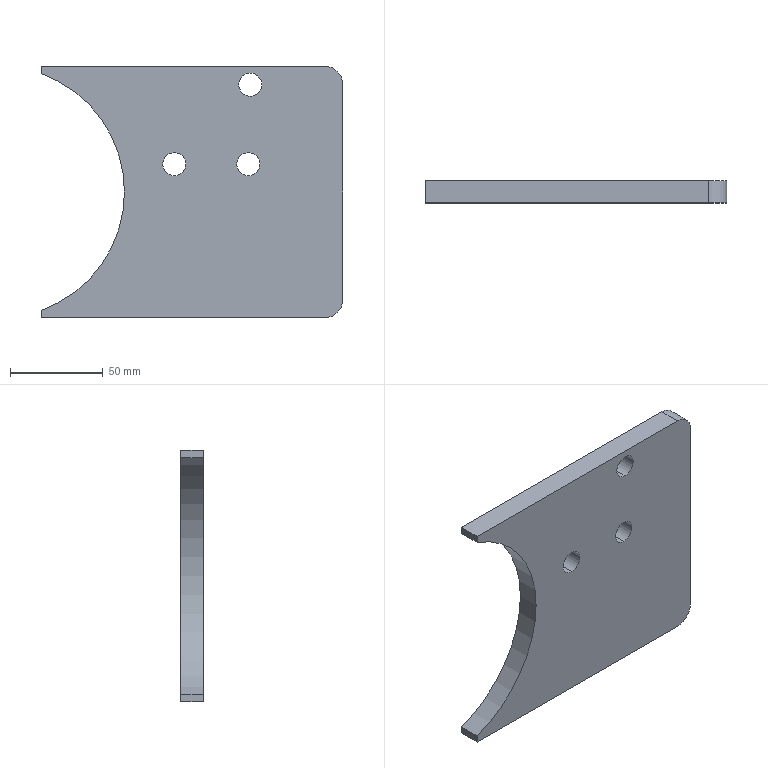Part | SolidWorks | features FlatPattern 1, SMBaseFlange 1, SheetMetal 1 | 1 solid | 16 faces | box 163 x 12 x 136 mm | volume 210730 mm3 | cylinder 9 | plane 7 | commonest cylinder face diameters 12.5 x6 20 x2 136 x1
STEP:
#1=CARTESIAN_POINT('',(113.,-12.,119.75));
#2=VERTEX_POINT('',#1);
#3=CARTESIAN_POINT('',(113.,-12.,132.25));
#4=VERTEX_POINT('',#3);
#5=CARTESIAN_POINT('',(113.,-12.,126.));
#6=DIRECTION('',(0.,1.,0.));
#7=DIRECTION('',(0.,0.,1.));
#8=AXIS2_PLACEMENT_3D('',#5,#6,#7);
#9=CIRCLE('',#8,6.25);
#10=EDGE_CURVE('',#2,#4,#9,.T.);
#11=ORIENTED_EDGE('',*,*,#10,.F.);
#12=CARTESIAN_POINT('',(113.,0.,119.75));
#13=VERTEX_POINT('',#12);
#14=CARTESIAN_POINT('',(113.,-12.,119.75));
#15=DIRECTION('',(0.,1.,0.));
#16=VECTOR('',#15,1000.);
#17=LINE('',#14,#16);
#18=EDGE_CURVE('',#2,#13,#17,.T.);
#19=ORIENTED_EDGE('',*,*,#18,.T.);
#20=CARTESIAN_POINT('',(113.,0.,132.25));
#21=VERTEX_POINT('',#20);
#22=CARTESIAN_POINT('',(113.,0.,126.));
#23=DIRECTION('',(0.,1.,0.));
#24=DIRECTION('',(0.,0.,1.));
#25=AXIS2_PLACEMENT_3D('',#22,#23,#24);
#26=CIRCLE('',#25,6.25);
#27=EDGE_CURVE('',#13,#21,#26,.T.);
#28=ORIENTED_EDGE('',*,*,#27,.T.);
#29=CARTESIAN_POINT('',(113.,-12.,132.25));
#30=DIRECTION('',(0.,1.,0.));
#31=VECTOR('',#30,1000.);
#32=LINE('',#29,#31);
#33=EDGE_CURVE('',#4,#21,#32,.T.);
#34=ORIENTED_EDGE('',*,*,#33,.F.);
#35=EDGE_LOOP('',(#11,#19,#28,#34));
#36=FACE_OUTER_BOUND('',#35,.T.);
#37=CARTESIAN_POINT('',(113.,-12.,126.));
#38=DIRECTION('',(0.,1.,0.));
#39=DIRECTION('',(0.,0.,1.));
#40=AXIS2_PLACEMENT_3D('',#37,#38,#39);
#41=CYLINDRICAL_SURFACE('',#40,6.25);
#42=ADVANCED_FACE('',(#36),#41,.F.);
#43=CARTESIAN_POINT('',(112.,-12.,76.75));
#44=VERTEX_POINT('',#43);
#45=CARTESIAN_POINT('',(112.,-12.,89.25));
#46=VERTEX_POINT('',#45);
#47=CARTESIAN_POINT('',(112.,-12.,83.));
#48=DIRECTION('',(0.,1.,0.));
#49=DIRECTION('',(0.,0.,1.));
#50=AXIS2_PLACEMENT_3D('',#47,#48,#49);
#51=CIRCLE('',#50,6.25);
#52=EDGE_CURVE('',#44,#46,#51,.T.);
#53=ORIENTED_EDGE('',*,*,#52,.F.);
#54=CARTESIAN_POINT('',(112.,0.,76.75));
#55=VERTEX_POINT('',#54);
#56=CARTESIAN_POINT('',(112.,-12.,76.75));
#57=DIRECTION('',(0.,1.,0.));
#58=VECTOR('',#57,1000.);
#59=LINE('',#56,#58);
#60=EDGE_CURVE('',#44,#55,#59,.T.);
#61=ORIENTED_EDGE('',*,*,#60,.T.);
#62=CARTESIAN_POINT('',(112.,0.,89.25));
#63=VERTEX_POINT('',#62);
#64=CARTESIAN_POINT('',(112.,0.,83.));
#65=DIRECTION('',(0.,1.,0.));
#66=DIRECTION('',(0.,0.,1.));
#67=AXIS2_PLACEMENT_3D('',#64,#65,#66);
#68=CIRCLE('',#67,6.25);
#69=EDGE_CURVE('',#55,#63,#68,.T.);
#70=ORIENTED_EDGE('',*,*,#69,.T.);
#71=CARTESIAN_POINT('',(112.,-12.,89.25));
#72=DIRECTION('',(0.,1.,0.));
#73=VECTOR('',#72,1000.);
#74=LINE('',#71,#73);
#75=EDGE_CURVE('',#46,#63,#74,.T.);
#76=ORIENTED_EDGE('',*,*,#75,.F.);
#77=EDGE_LOOP('',(#53,#61,#70,#76));
#78=FACE_OUTER_BOUND('',#77,.T.);
#79=CARTESIAN_POINT('',(112.,-12.,83.));
#80=DIRECTION('',(0.,1.,0.));
#81=DIRECTION('',(0.,0.,1.));
#82=AXIS2_PLACEMENT_3D('',#79,#80,#81);
#83=CYLINDRICAL_SURFACE('',#82,6.25);
#84=ADVANCED_FACE('',(#78),#83,.F.);
#85=CARTESIAN_POINT('',(72.,-12.,76.75));
#86=VERTEX_POINT('',#85);
#87=CARTESIAN_POINT('',(72.,-12.,89.25));
#88=VERTEX_POINT('',#87);
#89=CARTESIAN_POINT('',(72.,-12.,83.));
#90=DIRECTION('',(0.,1.,0.));
#91=DIRECTION('',(0.,0.,1.));
#92=AXIS2_PLACEMENT_3D('',#89,#90,#91);
#93=CIRCLE('',#92,6.25);
#94=EDGE_CURVE('',#86,#88,#93,.T.);
#95=ORIENTED_EDGE('',*,*,#94,.F.);
#96=CARTESIAN_POINT('',(72.,0.,76.75));
#97=VERTEX_POINT('',#96);
#98=CARTESIAN_POINT('',(72.,-12.,76.75));
#99=DIRECTION('',(0.,1.,0.));
#100=VECTOR('',#99,1000.);
#101=LINE('',#98,#100);
#102=EDGE_CURVE('',#86,#97,#101,.T.);
#103=ORIENTED_EDGE('',*,*,#102,.T.);
#104=CARTESIAN_POINT('',(72.,0.,89.25));
#105=VERTEX_POINT('',#104);
#106=CARTESIAN_POINT('',(72.,0.,83.));
#107=DIRECTION('',(0.,1.,0.));
#108=DIRECTION('',(0.,0.,1.));
#109=AXIS2_PLACEMENT_3D('',#106,#107,#108);
#110=CIRCLE('',#109,6.25);
#111=EDGE_CURVE('',#97,#105,#110,.T.);
#112=ORIENTED_EDGE('',*,*,#111,.T.);
#113=CARTESIAN_POINT('',(72.,-12.,89.25));
#114=DIRECTION('',(0.,1.,0.));
#115=VECTOR('',#114,1000.);
#116=LINE('',#113,#115);
#117=EDGE_CURVE('',#88,#105,#116,.T.);
#118=ORIENTED_EDGE('',*,*,#117,.F.);
#119=EDGE_LOOP('',(#95,#103,#112,#118));
#120=FACE_OUTER_BOUND('',#119,.T.);
#121=CARTESIAN_POINT('',(72.,-12.,83.));
#122=DIRECTION('',(0.,1.,0.));
#123=DIRECTION('',(0.,0.,1.));
#124=AXIS2_PLACEMENT_3D('',#121,#122,#123);
#125=CYLINDRICAL_SURFACE('',#124,6.25);
#126=ADVANCED_FACE('',(#120),#125,.F.);
#127=CARTESIAN_POINT('',(0.,0.,0.));
#128=VERTEX_POINT('',#127);
#129=CARTESIAN_POINT('',(0.,0.,4.008));
#130=VERTEX_POINT('',#129);
#131=CARTESIAN_POINT('',(0.,0.,0.));
#132=DIRECTION('',(0.,0.,1.));
#133=VECTOR('',#132,1000.);
#134=LINE('',#131,#133);
#135=EDGE_CURVE('',#128,#130,#134,.T.);
#136=ORIENTED_EDGE('',*,*,#135,.F.);
#137=CARTESIAN_POINT('',(0.,-12.,0.));
#138=VERTEX_POINT('',#137);
#139=CARTESIAN_POINT('',(0.,-12.,0.));
#140=DIRECTION('',(0.,1.,0.));
#141=VECTOR('',#140,1000.);
#142=LINE('',#139,#141);
#143=EDGE_CURVE('',#138,#128,#142,.T.);
#144=ORIENTED_EDGE('',*,*,#143,.F.);
#145=CARTESIAN_POINT('',(0.,-12.,4.008));
#146=VERTEX_POINT('',#145);
#147=CARTESIAN_POINT('',(0.,-12.,0.));
#148=DIRECTION('',(0.,0.,1.));
#149=VECTOR('',#148,1000.);
#150=LINE('',#147,#149);
#151=EDGE_CURVE('',#138,#146,#150,.T.);
#152=ORIENTED_EDGE('',*,*,#151,.T.);
#153=CARTESIAN_POINT('',(0.,-12.,4.008));
#154=DIRECTION('',(0.,1.,0.));
#155=VECTOR('',#154,1000.);
#156=LINE('',#153,#155);
#157=EDGE_CURVE('',#146,#130,#156,.T.);
#158=ORIENTED_EDGE('',*,*,#157,.T.);
#159=EDGE_LOOP('',(#136,#144,#152,#158));
#160=FACE_OUTER_BOUND('',#159,.T.);
#161=CARTESIAN_POINT('',(0.,-12.,0.));
#162=DIRECTION('',(-1.,0.,0.));
#163=DIRECTION('',(0.,0.,1.));
#164=AXIS2_PLACEMENT_3D('',#161,#162,#163);
#165=PLANE('',#164);
#166=ADVANCED_FACE('',(#160),#165,.T.);
#167=CARTESIAN_POINT('',(153.,0.,0.));
#168=VERTEX_POINT('',#167);
#169=CARTESIAN_POINT('',(0.,0.,0.));
#170=DIRECTION('',(-1.,0.,0.));
#171=VECTOR('',#170,1000.);
#172=LINE('',#169,#171);
#173=EDGE_CURVE('',#168,#128,#172,.T.);
#174=ORIENTED_EDGE('',*,*,#173,.F.);
#175=CARTESIAN_POINT('',(153.,-12.,0.));
#176=VERTEX_POINT('',#175);
#177=CARTESIAN_POINT('',(153.,-12.,0.));
#178=DIRECTION('',(0.,1.,0.));
#179=VECTOR('',#178,1000.);
#180=LINE('',#177,#179);
#181=EDGE_CURVE('',#176,#168,#180,.T.);
#182=ORIENTED_EDGE('',*,*,#181,.F.);
#183=CARTESIAN_POINT('',(0.,-12.,0.));
#184=DIRECTION('',(-1.,0.,0.));
#185=VECTOR('',#184,1000.);
#186=LINE('',#183,#185);
#187=EDGE_CURVE('',#176,#138,#186,.T.);
#188=ORIENTED_EDGE('',*,*,#187,.T.);
#189=ORIENTED_EDGE('',*,*,#143,.T.);
#190=EDGE_LOOP('',(#174,#182,#188,#189));
#191=FACE_OUTER_BOUND('',#190,.T.);
#192=CARTESIAN_POINT('',(0.,-12.,0.));
#193=DIRECTION('',(0.,0.,-1.));
#194=DIRECTION('',(-1.,0.,0.));
#195=AXIS2_PLACEMENT_3D('',#192,#193,#194);
#196=PLANE('',#195);
#197=ADVANCED_FACE('',(#191),#196,.T.);
#198=CARTESIAN_POINT('',(163.,0.,10.));
#199=VERTEX_POINT('',#198);
#200=CARTESIAN_POINT('',(153.,0.,10.));
#201=DIRECTION('',(0.,1.,0.));
#202=DIRECTION('',(0.,0.,-1.));
#203=AXIS2_PLACEMENT_3D('',#200,#201,#202);
#204=CIRCLE('',#203,10.);
#205=EDGE_CURVE('',#199,#168,#204,.T.);
#206=ORIENTED_EDGE('',*,*,#205,.F.);
#207=CARTESIAN_POINT('',(163.,-12.,10.));
#208=VERTEX_POINT('',#207);
#209=CARTESIAN_POINT('',(163.,-12.,10.));
#210=DIRECTION('',(0.,1.,0.));
#211=VECTOR('',#210,1000.);
#212=LINE('',#209,#211);
#213=EDGE_CURVE('',#208,#199,#212,.T.);
#214=ORIENTED_EDGE('',*,*,#213,.F.);
#215=CARTESIAN_POINT('',(153.,-12.,10.));
#216=DIRECTION('',(0.,1.,0.));
#217=DIRECTION('',(0.,0.,-1.));
#218=AXIS2_PLACEMENT_3D('',#215,#216,#217);
#219=CIRCLE('',#218,10.);
#220=EDGE_CURVE('',#208,#176,#219,.T.);
#221=ORIENTED_EDGE('',*,*,#220,.T.);
#222=ORIENTED_EDGE('',*,*,#181,.T.);
#223=EDGE_LOOP('',(#206,#214,#221,#222));
#224=FACE_OUTER_BOUND('',#223,.T.);
#225=CARTESIAN_POINT('',(153.,-12.,10.));
#226=DIRECTION('',(0.,1.,0.));
#227=DIRECTION('',(0.,0.,1.));
#228=AXIS2_PLACEMENT_3D('',#225,#226,#227);
#229=CYLINDRICAL_SURFACE('',#228,10.);
#230=ADVANCED_FACE('',(#224),#229,.T.);
#231=CARTESIAN_POINT('',(163.,0.,126.));
#232=VERTEX_POINT('',#231);
#233=CARTESIAN_POINT('',(163.,0.,10.));
#234=DIRECTION('',(0.,0.,-1.));
#235=VECTOR('',#234,1000.);
#236=LINE('',#233,#235);
#237=EDGE_CURVE('',#232,#199,#236,.T.);
#238=ORIENTED_EDGE('',*,*,#237,.F.);
#239=CARTESIAN_POINT('',(163.,-12.,126.));
#240=VERTEX_POINT('',#239);
#241=CARTESIAN_POINT('',(163.,-12.,126.));
#242=DIRECTION('',(0.,1.,0.));
#243=VECTOR('',#242,1000.);
#244=LINE('',#241,#243);
#245=EDGE_CURVE('',#240,#232,#244,.T.);
#246=ORIENTED_EDGE('',*,*,#245,.F.);
#247=CARTESIAN_POINT('',(163.,-12.,10.));
#248=DIRECTION('',(0.,0.,-1.));
#249=VECTOR('',#248,1000.);
#250=LINE('',#247,#249);
#251=EDGE_CURVE('',#240,#208,#250,.T.);
#252=ORIENTED_EDGE('',*,*,#251,.T.);
#253=ORIENTED_EDGE('',*,*,#213,.T.);
#254=EDGE_LOOP('',(#238,#246,#252,#253));
#255=FACE_OUTER_BOUND('',#254,.T.);
#256=CARTESIAN_POINT('',(163.,-12.,10.));
#257=DIRECTION('',(1.,0.,0.));
#258=DIRECTION('',(0.,0.,-1.));
#259=AXIS2_PLACEMENT_3D('',#256,#257,#258);
#260=PLANE('',#259);
#261=ADVANCED_FACE('',(#255),#260,.T.);
#262=CARTESIAN_POINT('',(153.,0.,136.));
#263=VERTEX_POINT('',#262);
#264=CARTESIAN_POINT('',(153.,0.,126.));
#265=DIRECTION('',(0.,1.,0.));
#266=DIRECTION('',(0.,0.,1.));
#267=AXIS2_PLACEMENT_3D('',#264,#265,#266);
#268=CIRCLE('',#267,10.);
#269=EDGE_CURVE('',#263,#232,#268,.T.);
#270=ORIENTED_EDGE('',*,*,#269,.F.);
#271=CARTESIAN_POINT('',(153.,-12.,136.));
#272=VERTEX_POINT('',#271);
#273=CARTESIAN_POINT('',(153.,-12.,136.));
#274=DIRECTION('',(0.,1.,0.));
#275=VECTOR('',#274,1000.);
#276=LINE('',#273,#275);
#277=EDGE_CURVE('',#272,#263,#276,.T.);
#278=ORIENTED_EDGE('',*,*,#277,.F.);
#279=CARTESIAN_POINT('',(153.,-12.,126.));
#280=DIRECTION('',(0.,1.,0.));
#281=DIRECTION('',(0.,0.,1.));
#282=AXIS2_PLACEMENT_3D('',#279,#280,#281);
#283=CIRCLE('',#282,10.);
#284=EDGE_CURVE('',#272,#240,#283,.T.);
#285=ORIENTED_EDGE('',*,*,#284,.T.);
#286=ORIENTED_EDGE('',*,*,#245,.T.);
#287=EDGE_LOOP('',(#270,#278,#285,#286));
#288=FACE_OUTER_BOUND('',#287,.T.);
#289=CARTESIAN_POINT('',(153.,-12.,126.));
#290=DIRECTION('',(0.,1.,0.));
#291=DIRECTION('',(0.,0.,1.));
#292=AXIS2_PLACEMENT_3D('',#289,#290,#291);
#293=CYLINDRICAL_SURFACE('',#292,10.);
#294=ADVANCED_FACE('',(#288),#293,.T.);
#295=CARTESIAN_POINT('',(0.,0.,136.));
#296=VERTEX_POINT('',#295);
#297=CARTESIAN_POINT('',(0.,0.,136.));
#298=DIRECTION('',(1.,0.,0.));
#299=VECTOR('',#298,1000.);
#300=LINE('',#297,#299);
#301=EDGE_CURVE('',#296,#263,#300,.T.);
#302=ORIENTED_EDGE('',*,*,#301,.F.);
#303=CARTESIAN_POINT('',(0.,-12.,136.));
#304=VERTEX_POINT('',#303);
#305=CARTESIAN_POINT('',(0.,-12.,136.));
#306=DIRECTION('',(0.,1.,0.));
#307=VECTOR('',#306,1000.);
#308=LINE('',#305,#307);
#309=EDGE_CURVE('',#304,#296,#308,.T.);
#310=ORIENTED_EDGE('',*,*,#309,.F.);
#311=CARTESIAN_POINT('',(0.,-12.,136.));
#312=DIRECTION('',(1.,0.,0.));
#313=VECTOR('',#312,1000.);
#314=LINE('',#311,#313);
#315=EDGE_CURVE('',#304,#272,#314,.T.);
#316=ORIENTED_EDGE('',*,*,#315,.T.);
#317=ORIENTED_EDGE('',*,*,#277,.T.);
#318=EDGE_LOOP('',(#302,#310,#316,#317));
#319=FACE_OUTER_BOUND('',#318,.T.);
#320=CARTESIAN_POINT('',(0.,-12.,136.));
#321=DIRECTION('',(0.,0.,1.));
#322=DIRECTION('',(1.,0.,0.));
#323=AXIS2_PLACEMENT_3D('',#320,#321,#322);
#324=PLANE('',#323);
#325=ADVANCED_FACE('',(#319),#324,.T.);
#326=CARTESIAN_POINT('',(0.,0.,131.992));
#327=VERTEX_POINT('',#326);
#328=CARTESIAN_POINT('',(0.,0.,131.992));
#329=DIRECTION('',(0.,0.,1.));
#330=VECTOR('',#329,1000.);
#331=LINE('',#328,#330);
#332=EDGE_CURVE('',#327,#296,#331,.T.);
#333=ORIENTED_EDGE('',*,*,#332,.F.);
#334=CARTESIAN_POINT('',(0.,-12.,131.992));
#335=VERTEX_POINT('',#334);
#336=CARTESIAN_POINT('',(0.,-12.,131.992));
#337=DIRECTION('',(0.,1.,0.));
#338=VECTOR('',#337,1000.);
#339=LINE('',#336,#338);
#340=EDGE_CURVE('',#335,#327,#339,.T.);
#341=ORIENTED_EDGE('',*,*,#340,.F.);
#342=CARTESIAN_POINT('',(0.,-12.,131.992));
#343=DIRECTION('',(0.,0.,1.));
#344=VECTOR('',#343,1000.);
#345=LINE('',#342,#344);
#346=EDGE_CURVE('',#335,#304,#345,.T.);
#347=ORIENTED_EDGE('',*,*,#346,.T.);
#348=ORIENTED_EDGE('',*,*,#309,.T.);
#349=EDGE_LOOP('',(#333,#341,#347,#348));
#350=FACE_OUTER_BOUND('',#349,.T.);
#351=CARTESIAN_POINT('',(0.,-12.,131.992));
#352=DIRECTION('',(-1.,0.,0.));
#353=DIRECTION('',(0.,0.,1.));
#354=AXIS2_PLACEMENT_3D('',#351,#352,#353);
#355=PLANE('',#354);
#356=ADVANCED_FACE('',(#350),#355,.T.);
#357=CARTESIAN_POINT('',(-23.,0.,68.));
#358=DIRECTION('',(0.,-1.,0.));
#359=DIRECTION('',(0.,0.,1.));
#360=AXIS2_PLACEMENT_3D('',#357,#358,#359);
#361=CIRCLE('',#360,68.);
#362=EDGE_CURVE('',#130,#327,#361,.T.);
#363=ORIENTED_EDGE('',*,*,#362,.F.);
#364=ORIENTED_EDGE('',*,*,#157,.F.);
#365=CARTESIAN_POINT('',(-23.,-12.,68.));
#366=DIRECTION('',(0.,-1.,0.));
#367=DIRECTION('',(0.,0.,1.));
#368=AXIS2_PLACEMENT_3D('',#365,#366,#367);
#369=CIRCLE('',#368,68.);
#370=EDGE_CURVE('',#146,#335,#369,.T.);
#371=ORIENTED_EDGE('',*,*,#370,.T.);
#372=ORIENTED_EDGE('',*,*,#340,.T.);
#373=EDGE_LOOP('',(#363,#364,#371,#372));
#374=FACE_OUTER_BOUND('',#373,.T.);
#375=CARTESIAN_POINT('',(-23.,-12.,68.));
#376=DIRECTION('',(0.,1.,0.));
#377=DIRECTION('',(0.,0.,1.));
#378=AXIS2_PLACEMENT_3D('',#375,#376,#377);
#379=CYLINDRICAL_SURFACE('',#378,68.);
#380=ADVANCED_FACE('',(#374),#379,.F.);
#381=CARTESIAN_POINT('',(113.,-12.,126.));
#382=DIRECTION('',(0.,1.,0.));
#383=DIRECTION('',(0.,0.,1.));
#384=AXIS2_PLACEMENT_3D('',#381,#382,#383);
#385=CIRCLE('',#384,6.25);
#386=EDGE_CURVE('',#4,#2,#385,.T.);
#387=ORIENTED_EDGE('',*,*,#386,.T.);
#388=ORIENTED_EDGE('',*,*,#10,.T.);
#389=EDGE_LOOP('',(#387,#388));
#390=FACE_BOUND('',#389,.T.);
#391=CARTESIAN_POINT('',(112.,-12.,83.));
#392=DIRECTION('',(0.,1.,0.));
#393=DIRECTION('',(0.,0.,1.));
#394=AXIS2_PLACEMENT_3D('',#391,#392,#393);
#395=CIRCLE('',#394,6.25);
#396=EDGE_CURVE('',#46,#44,#395,.T.);
#397=ORIENTED_EDGE('',*,*,#396,.T.);
#398=ORIENTED_EDGE('',*,*,#52,.T.);
#399=EDGE_LOOP('',(#397,#398));
#400=FACE_BOUND('',#399,.T.);
#401=CARTESIAN_POINT('',(72.,-12.,83.));
#402=DIRECTION('',(0.,1.,0.));
#403=DIRECTION('',(0.,0.,1.));
#404=AXIS2_PLACEMENT_3D('',#401,#402,#403);
#405=CIRCLE('',#404,6.25);
#406=EDGE_CURVE('',#88,#86,#405,.T.);
#407=ORIENTED_EDGE('',*,*,#406,.T.);
#408=ORIENTED_EDGE('',*,*,#94,.T.);
#409=EDGE_LOOP('',(#407,#408));
#410=FACE_BOUND('',#409,.T.);
#411=ORIENTED_EDGE('',*,*,#151,.F.);
#412=ORIENTED_EDGE('',*,*,#187,.F.);
#413=ORIENTED_EDGE('',*,*,#220,.F.);
#414=ORIENTED_EDGE('',*,*,#251,.F.);
#415=ORIENTED_EDGE('',*,*,#284,.F.);
#416=ORIENTED_EDGE('',*,*,#315,.F.);
#417=ORIENTED_EDGE('',*,*,#346,.F.);
#418=ORIENTED_EDGE('',*,*,#370,.F.);
#419=EDGE_LOOP('',(#411,#412,#413,#414,#415,#416,#417,#418));
#420=FACE_OUTER_BOUND('',#419,.T.);
#421=CARTESIAN_POINT('',(-23.,-12.,68.));
#422=DIRECTION('',(0.,1.,0.));
#423=DIRECTION('',(0.,0.,1.));
#424=AXIS2_PLACEMENT_3D('',#421,#422,#423);
#425=PLANE('',#424);
#426=ADVANCED_FACE('',(#390,#400,#410,#420),#425,.F.);
#427=CARTESIAN_POINT('',(113.,0.,126.));
#428=DIRECTION('',(0.,1.,0.));
#429=DIRECTION('',(0.,0.,1.));
#430=AXIS2_PLACEMENT_3D('',#427,#428,#429);
#431=CIRCLE('',#430,6.25);
#432=EDGE_CURVE('',#21,#13,#431,.T.);
#433=ORIENTED_EDGE('',*,*,#432,.F.);
#434=ORIENTED_EDGE('',*,*,#27,.F.);
#435=EDGE_LOOP('',(#433,#434));
#436=FACE_BOUND('',#435,.T.);
#437=CARTESIAN_POINT('',(112.,0.,83.));
#438=DIRECTION('',(0.,1.,0.));
#439=DIRECTION('',(0.,0.,1.));
#440=AXIS2_PLACEMENT_3D('',#437,#438,#439);
#441=CIRCLE('',#440,6.25);
#442=EDGE_CURVE('',#63,#55,#441,.T.);
#443=ORIENTED_EDGE('',*,*,#442,.F.);
#444=ORIENTED_EDGE('',*,*,#69,.F.);
#445=EDGE_LOOP('',(#443,#444));
#446=FACE_BOUND('',#445,.T.);
#447=CARTESIAN_POINT('',(72.,0.,83.));
#448=DIRECTION('',(0.,1.,0.));
#449=DIRECTION('',(0.,0.,1.));
#450=AXIS2_PLACEMENT_3D('',#447,#448,#449);
#451=CIRCLE('',#450,6.25);
#452=EDGE_CURVE('',#105,#97,#451,.T.);
#453=ORIENTED_EDGE('',*,*,#452,.F.);
#454=ORIENTED_EDGE('',*,*,#111,.F.);
#455=EDGE_LOOP('',(#453,#454));
#456=FACE_BOUND('',#455,.T.);
#457=ORIENTED_EDGE('',*,*,#135,.T.);
#458=ORIENTED_EDGE('',*,*,#362,.T.);
#459=ORIENTED_EDGE('',*,*,#332,.T.);
#460=ORIENTED_EDGE('',*,*,#301,.T.);
#461=ORIENTED_EDGE('',*,*,#269,.T.);
#462=ORIENTED_EDGE('',*,*,#237,.T.);
#463=ORIENTED_EDGE('',*,*,#205,.T.);
#464=ORIENTED_EDGE('',*,*,#173,.T.);
#465=EDGE_LOOP('',(#457,#458,#459,#460,#461,#462,#463,#464));
#466=FACE_OUTER_BOUND('',#465,.T.);
#467=CARTESIAN_POINT('',(-23.,0.,68.));
#468=DIRECTION('',(0.,1.,0.));
#469=DIRECTION('',(0.,0.,1.));
#470=AXIS2_PLACEMENT_3D('',#467,#468,#469);
#471=PLANE('',#470);
#472=ADVANCED_FACE('',(#436,#446,#456,#466),#471,.T.);
#473=ORIENTED_EDGE('',*,*,#102,.F.);
#474=ORIENTED_EDGE('',*,*,#406,.F.);
#475=ORIENTED_EDGE('',*,*,#117,.T.);
#476=ORIENTED_EDGE('',*,*,#452,.T.);
#477=EDGE_LOOP('',(#473,#474,#475,#476));
#478=FACE_OUTER_BOUND('',#477,.T.);
#479=CARTESIAN_POINT('',(72.,-12.,83.));
#480=DIRECTION('',(0.,1.,0.));
#481=DIRECTION('',(0.,0.,1.));
#482=AXIS2_PLACEMENT_3D('',#479,#480,#481);
#483=CYLINDRICAL_SURFACE('',#482,6.25);
#484=ADVANCED_FACE('',(#478),#483,.F.);
#485=ORIENTED_EDGE('',*,*,#60,.F.);
#486=ORIENTED_EDGE('',*,*,#396,.F.);
#487=ORIENTED_EDGE('',*,*,#75,.T.);
#488=ORIENTED_EDGE('',*,*,#442,.T.);
#489=EDGE_LOOP('',(#485,#486,#487,#488));
#490=FACE_OUTER_BOUND('',#489,.T.);
#491=CARTESIAN_POINT('',(112.,-12.,83.));
#492=DIRECTION('',(0.,1.,0.));
#493=DIRECTION('',(0.,0.,1.));
#494=AXIS2_PLACEMENT_3D('',#491,#492,#493);
#495=CYLINDRICAL_SURFACE('',#494,6.25);
#496=ADVANCED_FACE('',(#490),#495,.F.);
#497=ORIENTED_EDGE('',*,*,#18,.F.);
#498=ORIENTED_EDGE('',*,*,#386,.F.);
#499=ORIENTED_EDGE('',*,*,#33,.T.);
#500=ORIENTED_EDGE('',*,*,#432,.T.);
#501=EDGE_LOOP('',(#497,#498,#499,#500));
#502=FACE_OUTER_BOUND('',#501,.T.);
#503=CARTESIAN_POINT('',(113.,-12.,126.));
#504=DIRECTION('',(0.,1.,0.));
#505=DIRECTION('',(0.,0.,1.));
#506=AXIS2_PLACEMENT_3D('',#503,#504,#505);
#507=CYLINDRICAL_SURFACE('',#506,6.25);
#508=ADVANCED_FACE('',(#502),#507,.F.);
#509=CLOSED_SHELL('',(#42,#84,#126,#166,#197,#230,#261,#294,#325,#356,#380,#426,#472,#484,#496,#508));
#510=MANIFOLD_SOLID_BREP('',#509);
#511=CARTESIAN_POINT('',(0.,0.,0.));
#512=DIRECTION('',(0.,0.,1.));
#513=DIRECTION('',(1.,0.,0.));
#514=AXIS2_PLACEMENT_3D('',#511,#512,#513);
#515=(LENGTH_UNIT()NAMED_UNIT(*)SI_UNIT(.MILLI.,.METRE.));
#516=UNCERTAINTY_MEASURE_WITH_UNIT(LENGTH_MEASURE(0.00001),#515,'','');
#517=(NAMED_UNIT(*)PLANE_ANGLE_UNIT()SI_UNIT($,.RADIAN.));
#518=(NAMED_UNIT(*)SI_UNIT($,.STERADIAN.)SOLID_ANGLE_UNIT());
#519=(GEOMETRIC_REPRESENTATION_CONTEXT(3)GLOBAL_UNCERTAINTY_ASSIGNED_CONTEXT((#516))GLOBAL_UNIT_ASSIGNED_CONTEXT((#515,#517,#518))REPRESENTATION_CONTEXT('',''));
#520=ADVANCED_BREP_SHAPE_REPRESENTATION('',(#510,#514),#519);